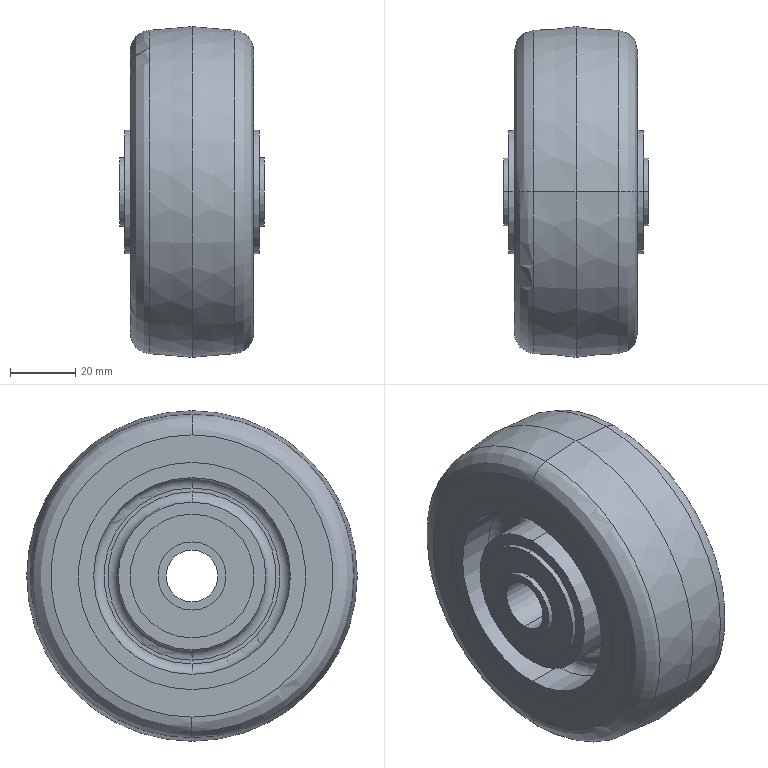Part | SolidWorks | features Revolution 1 | 1 solid | 56 faces | box 44.45 x 101.6 x 101.6 mm | volume 249789 mm3 | cylinder 26 | plane 14 | torus 12 | cone 4 | commonest cylinder face diameters 15.85 x4 20.955 x4 38.1 x4 45.415 x4 60.452 x4 69.85 x4
STEP:
#1=CARTESIAN_POINT('',(-0.375,0.,-0.312));
#2=VERTEX_POINT('',#1);
#3=CARTESIAN_POINT('',(-0.375,0.,0.312));
#4=VERTEX_POINT('',#3);
#5=CARTESIAN_POINT('',(-0.375,0.,0.));
#6=DIRECTION('',(-1.,0.,0.));
#7=DIRECTION('',(0.,0.,1.));
#8=AXIS2_PLACEMENT_3D('',#5,#6,#7);
#9=CIRCLE('',#8,0.312);
#10=EDGE_CURVE('',#2,#4,#9,.T.);
#11=ORIENTED_EDGE('',*,*,#10,.F.);
#12=CARTESIAN_POINT('',(-0.875,0.,-0.312));
#13=VERTEX_POINT('',#12);
#14=CARTESIAN_POINT('',(-1.26,0.,-0.312));
#15=DIRECTION('',(-1.,0.,0.));
#16=VECTOR('',#15,39.37);
#17=LINE('',#14,#16);
#18=EDGE_CURVE('',#2,#13,#17,.T.);
#19=ORIENTED_EDGE('',*,*,#18,.T.);
#20=CARTESIAN_POINT('',(-0.875,0.,0.312));
#21=VERTEX_POINT('',#20);
#22=CARTESIAN_POINT('',(-0.875,0.,0.));
#23=DIRECTION('',(-1.,0.,0.));
#24=DIRECTION('',(0.,0.,1.));
#25=AXIS2_PLACEMENT_3D('',#22,#23,#24);
#26=CIRCLE('',#25,0.312);
#27=EDGE_CURVE('',#13,#21,#26,.T.);
#28=ORIENTED_EDGE('',*,*,#27,.T.);
#29=CARTESIAN_POINT('',(-1.26,0.,0.312));
#30=DIRECTION('',(-1.,0.,0.));
#31=VECTOR('',#30,39.37);
#32=LINE('',#29,#31);
#33=EDGE_CURVE('',#4,#21,#32,.T.);
#34=ORIENTED_EDGE('',*,*,#33,.F.);
#35=EDGE_LOOP('',(#11,#19,#28,#34));
#36=FACE_OUTER_BOUND('',#35,.T.);
#37=CARTESIAN_POINT('',(-1.26,0.,0.));
#38=DIRECTION('',(-1.,0.,0.));
#39=DIRECTION('',(0.,0.,1.));
#40=AXIS2_PLACEMENT_3D('',#37,#38,#39);
#41=CYLINDRICAL_SURFACE('',#40,0.312);
#42=ADVANCED_FACE('',(#36),#41,.F.);
#43=CARTESIAN_POINT('',(-0.8125,0.,0.4125));
#44=VERTEX_POINT('',#43);
#45=CARTESIAN_POINT('',(-0.8125,0.,-0.4125));
#46=VERTEX_POINT('',#45);
#47=CARTESIAN_POINT('',(-0.8125,0.,0.));
#48=DIRECTION('',(-1.,0.,0.));
#49=DIRECTION('',(0.,0.,1.));
#50=AXIS2_PLACEMENT_3D('',#47,#48,#49);
#51=CIRCLE('',#50,0.4125);
#52=EDGE_CURVE('',#44,#46,#51,.T.);
#53=ORIENTED_EDGE('',*,*,#52,.T.);
#54=CARTESIAN_POINT('',(-0.875,0.,-0.4125));
#55=VERTEX_POINT('',#54);
#56=CARTESIAN_POINT('',(-1.26,0.,-0.4125));
#57=DIRECTION('',(-1.,0.,0.));
#58=VECTOR('',#57,39.37);
#59=LINE('',#56,#58);
#60=EDGE_CURVE('',#46,#55,#59,.T.);
#61=ORIENTED_EDGE('',*,*,#60,.T.);
#62=CARTESIAN_POINT('',(-0.875,0.,0.4125));
#63=VERTEX_POINT('',#62);
#64=CARTESIAN_POINT('',(-0.875,0.,0.));
#65=DIRECTION('',(-1.,0.,0.));
#66=DIRECTION('',(0.,0.,1.));
#67=AXIS2_PLACEMENT_3D('',#64,#65,#66);
#68=CIRCLE('',#67,0.4125);
#69=EDGE_CURVE('',#63,#55,#68,.T.);
#70=ORIENTED_EDGE('',*,*,#69,.F.);
#71=CARTESIAN_POINT('',(-1.26,0.,0.4125));
#72=DIRECTION('',(-1.,0.,0.));
#73=VECTOR('',#72,39.37);
#74=LINE('',#71,#73);
#75=EDGE_CURVE('',#44,#63,#74,.T.);
#76=ORIENTED_EDGE('',*,*,#75,.F.);
#77=EDGE_LOOP('',(#53,#61,#70,#76));
#78=FACE_OUTER_BOUND('',#77,.T.);
#79=CARTESIAN_POINT('',(-1.26,0.,0.));
#80=DIRECTION('',(-1.,0.,0.));
#81=DIRECTION('',(0.,0.,1.));
#82=AXIS2_PLACEMENT_3D('',#79,#80,#81);
#83=CYLINDRICAL_SURFACE('',#82,0.4125);
#84=ADVANCED_FACE('',(#78),#83,.T.);
#85=CARTESIAN_POINT('',(-0.75,0.,0.75));
#86=VERTEX_POINT('',#85);
#87=CARTESIAN_POINT('',(-0.75,0.,-0.75));
#88=VERTEX_POINT('',#87);
#89=CARTESIAN_POINT('',(-0.75,0.,0.));
#90=DIRECTION('',(-1.,0.,0.));
#91=DIRECTION('',(0.,0.,1.));
#92=AXIS2_PLACEMENT_3D('',#89,#90,#91);
#93=CIRCLE('',#92,0.75);
#94=EDGE_CURVE('',#86,#88,#93,.T.);
#95=ORIENTED_EDGE('',*,*,#94,.T.);
#96=CARTESIAN_POINT('',(-0.8125,0.,-0.75));
#97=VERTEX_POINT('',#96);
#98=CARTESIAN_POINT('',(-1.26,0.,-0.75));
#99=DIRECTION('',(-1.,0.,0.));
#100=VECTOR('',#99,39.37);
#101=LINE('',#98,#100);
#102=EDGE_CURVE('',#88,#97,#101,.T.);
#103=ORIENTED_EDGE('',*,*,#102,.T.);
#104=CARTESIAN_POINT('',(-0.8125,0.,0.75));
#105=VERTEX_POINT('',#104);
#106=CARTESIAN_POINT('',(-0.8125,0.,0.));
#107=DIRECTION('',(-1.,0.,0.));
#108=DIRECTION('',(0.,0.,1.));
#109=AXIS2_PLACEMENT_3D('',#106,#107,#108);
#110=CIRCLE('',#109,0.75);
#111=EDGE_CURVE('',#105,#97,#110,.T.);
#112=ORIENTED_EDGE('',*,*,#111,.F.);
#113=CARTESIAN_POINT('',(-1.26,0.,0.75));
#114=DIRECTION('',(-1.,0.,0.));
#115=VECTOR('',#114,39.37);
#116=LINE('',#113,#115);
#117=EDGE_CURVE('',#86,#105,#116,.T.);
#118=ORIENTED_EDGE('',*,*,#117,.F.);
#119=EDGE_LOOP('',(#95,#103,#112,#118));
#120=FACE_OUTER_BOUND('',#119,.T.);
#121=CARTESIAN_POINT('',(-1.26,0.,0.));
#122=DIRECTION('',(-1.,0.,0.));
#123=DIRECTION('',(0.,0.,1.));
#124=AXIS2_PLACEMENT_3D('',#121,#122,#123);
#125=CYLINDRICAL_SURFACE('',#124,0.75);
#126=ADVANCED_FACE('',(#120),#125,.T.);
#127=CARTESIAN_POINT('',(-0.3125,0.,0.894));
#128=VERTEX_POINT('',#127);
#129=CARTESIAN_POINT('',(-0.3125,0.,-0.894));
#130=VERTEX_POINT('',#129);
#131=CARTESIAN_POINT('',(-0.3125,0.,0.));
#132=DIRECTION('',(-1.,0.,0.));
#133=DIRECTION('',(0.,0.,1.));
#134=AXIS2_PLACEMENT_3D('',#131,#132,#133);
#135=CIRCLE('',#134,0.894);
#136=EDGE_CURVE('',#128,#130,#135,.T.);
#137=ORIENTED_EDGE('',*,*,#136,.T.);
#138=CARTESIAN_POINT('',(-0.75,0.,-0.894));
#139=VERTEX_POINT('',#138);
#140=CARTESIAN_POINT('',(-1.26,0.,-0.894));
#141=DIRECTION('',(-1.,0.,0.));
#142=VECTOR('',#141,39.37);
#143=LINE('',#140,#142);
#144=EDGE_CURVE('',#130,#139,#143,.T.);
#145=ORIENTED_EDGE('',*,*,#144,.T.);
#146=CARTESIAN_POINT('',(-0.75,0.,0.894));
#147=VERTEX_POINT('',#146);
#148=CARTESIAN_POINT('',(-0.75,0.,0.));
#149=DIRECTION('',(-1.,0.,0.));
#150=DIRECTION('',(0.,0.,1.));
#151=AXIS2_PLACEMENT_3D('',#148,#149,#150);
#152=CIRCLE('',#151,0.894);
#153=EDGE_CURVE('',#147,#139,#152,.T.);
#154=ORIENTED_EDGE('',*,*,#153,.F.);
#155=CARTESIAN_POINT('',(-1.26,0.,0.894));
#156=DIRECTION('',(-1.,0.,0.));
#157=VECTOR('',#156,39.37);
#158=LINE('',#155,#157);
#159=EDGE_CURVE('',#128,#147,#158,.T.);
#160=ORIENTED_EDGE('',*,*,#159,.F.);
#161=EDGE_LOOP('',(#137,#145,#154,#160));
#162=FACE_OUTER_BOUND('',#161,.T.);
#163=CARTESIAN_POINT('',(-1.26,0.,0.));
#164=DIRECTION('',(-1.,0.,0.));
#165=DIRECTION('',(0.,0.,1.));
#166=AXIS2_PLACEMENT_3D('',#163,#164,#165);
#167=CYLINDRICAL_SURFACE('',#166,0.894);
#168=ADVANCED_FACE('',(#162),#167,.T.);
#169=CARTESIAN_POINT('',(-0.3125,0.,0.));
#170=DIRECTION('',(-1.,0.,0.));
#171=DIRECTION('',(0.,0.,1.));
#172=AXIS2_PLACEMENT_3D('',#169,#170,#171);
#173=CIRCLE('',#172,0.894);
#174=EDGE_CURVE('',#130,#128,#173,.T.);
#175=ORIENTED_EDGE('',*,*,#174,.F.);
#176=CARTESIAN_POINT('',(-0.1875,0.,-1.019));
#177=VERTEX_POINT('',#176);
#178=CARTESIAN_POINT('',(-0.3125,0.,-1.019));
#179=DIRECTION('',(0.,1.,0.));
#180=DIRECTION('',(0.,0.,1.));
#181=AXIS2_PLACEMENT_3D('',#178,#179,#180);
#182=CIRCLE('',#181,0.125);
#183=EDGE_CURVE('',#130,#177,#182,.T.);
#184=ORIENTED_EDGE('',*,*,#183,.T.);
#185=CARTESIAN_POINT('',(-0.1875,0.,1.019));
#186=VERTEX_POINT('',#185);
#187=CARTESIAN_POINT('',(-0.1875,0.,0.));
#188=DIRECTION('',(-1.,0.,0.));
#189=DIRECTION('',(0.,0.,1.));
#190=AXIS2_PLACEMENT_3D('',#187,#188,#189);
#191=CIRCLE('',#190,1.019);
#192=EDGE_CURVE('',#177,#186,#191,.T.);
#193=ORIENTED_EDGE('',*,*,#192,.T.);
#194=CARTESIAN_POINT('',(-0.3125,0.,1.019));
#195=DIRECTION('',(0.,-1.,0.));
#196=DIRECTION('',(0.,0.,-1.));
#197=AXIS2_PLACEMENT_3D('',#194,#195,#196);
#198=CIRCLE('',#197,0.125);
#199=EDGE_CURVE('',#128,#186,#198,.T.);
#200=ORIENTED_EDGE('',*,*,#199,.F.);
#201=EDGE_LOOP('',(#175,#184,#193,#200));
#202=FACE_OUTER_BOUND('',#201,.T.);
#203=CARTESIAN_POINT('',(-0.3125,0.,0.));
#204=DIRECTION('',(-1.,0.,0.));
#205=DIRECTION('',(0.,0.,1.));
#206=AXIS2_PLACEMENT_3D('',#203,#204,#205);
#207=TOROIDAL_SURFACE('',#206,1.019,0.125);
#208=ADVANCED_FACE('',(#202),#207,.F.);
#209=CARTESIAN_POINT('',(-0.1875,0.,-1.065));
#210=VERTEX_POINT('',#209);
#211=CARTESIAN_POINT('',(-0.1875,0.,1.065));
#212=VERTEX_POINT('',#211);
#213=CARTESIAN_POINT('',(-0.1875,0.,0.));
#214=DIRECTION('',(-1.,0.,0.));
#215=DIRECTION('',(0.,0.,1.));
#216=AXIS2_PLACEMENT_3D('',#213,#214,#215);
#217=CIRCLE('',#216,1.065);
#218=EDGE_CURVE('',#210,#212,#217,.T.);
#219=ORIENTED_EDGE('',*,*,#218,.F.);
#220=CARTESIAN_POINT('',(-0.3125,0.,-1.19));
#221=VERTEX_POINT('',#220);
#222=CARTESIAN_POINT('',(-0.3125,0.,-1.065));
#223=DIRECTION('',(0.,1.,0.));
#224=DIRECTION('',(0.,0.,1.));
#225=AXIS2_PLACEMENT_3D('',#222,#223,#224);
#226=CIRCLE('',#225,0.125);
#227=EDGE_CURVE('',#210,#221,#226,.T.);
#228=ORIENTED_EDGE('',*,*,#227,.T.);
#229=CARTESIAN_POINT('',(-0.3125,0.,1.19));
#230=VERTEX_POINT('',#229);
#231=CARTESIAN_POINT('',(-0.3125,0.,0.));
#232=DIRECTION('',(-1.,0.,0.));
#233=DIRECTION('',(0.,0.,1.));
#234=AXIS2_PLACEMENT_3D('',#231,#232,#233);
#235=CIRCLE('',#234,1.19);
#236=EDGE_CURVE('',#221,#230,#235,.T.);
#237=ORIENTED_EDGE('',*,*,#236,.T.);
#238=CARTESIAN_POINT('',(-0.3125,0.,1.065));
#239=DIRECTION('',(0.,-1.,0.));
#240=DIRECTION('',(0.,0.,-1.));
#241=AXIS2_PLACEMENT_3D('',#238,#239,#240);
#242=CIRCLE('',#241,0.125);
#243=EDGE_CURVE('',#212,#230,#242,.T.);
#244=ORIENTED_EDGE('',*,*,#243,.F.);
#245=EDGE_LOOP('',(#219,#228,#237,#244));
#246=FACE_OUTER_BOUND('',#245,.T.);
#247=CARTESIAN_POINT('',(-0.3125,0.,0.));
#248=DIRECTION('',(-1.,0.,0.));
#249=DIRECTION('',(0.,0.,1.));
#250=AXIS2_PLACEMENT_3D('',#247,#248,#249);
#251=TOROIDAL_SURFACE('',#250,1.065,0.125);
#252=ADVANCED_FACE('',(#246),#251,.F.);
#253=ORIENTED_EDGE('',*,*,#236,.F.);
#254=CARTESIAN_POINT('',(-0.75,0.,-1.19));
#255=VERTEX_POINT('',#254);
#256=CARTESIAN_POINT('',(-1.26,0.,-1.19));
#257=DIRECTION('',(-1.,0.,0.));
#258=VECTOR('',#257,39.37);
#259=LINE('',#256,#258);
#260=EDGE_CURVE('',#221,#255,#259,.T.);
#261=ORIENTED_EDGE('',*,*,#260,.T.);
#262=CARTESIAN_POINT('',(-0.75,0.,1.19));
#263=VERTEX_POINT('',#262);
#264=CARTESIAN_POINT('',(-0.75,0.,0.));
#265=DIRECTION('',(-1.,0.,0.));
#266=DIRECTION('',(0.,0.,1.));
#267=AXIS2_PLACEMENT_3D('',#264,#265,#266);
#268=CIRCLE('',#267,1.19);
#269=EDGE_CURVE('',#255,#263,#268,.T.);
#270=ORIENTED_EDGE('',*,*,#269,.T.);
#271=CARTESIAN_POINT('',(-1.26,0.,1.19));
#272=DIRECTION('',(-1.,0.,0.));
#273=VECTOR('',#272,39.37);
#274=LINE('',#271,#273);
#275=EDGE_CURVE('',#230,#263,#274,.T.);
#276=ORIENTED_EDGE('',*,*,#275,.F.);
#277=EDGE_LOOP('',(#253,#261,#270,#276));
#278=FACE_OUTER_BOUND('',#277,.T.);
#279=CARTESIAN_POINT('',(-1.26,0.,0.));
#280=DIRECTION('',(-1.,0.,0.));
#281=DIRECTION('',(0.,0.,1.));
#282=AXIS2_PLACEMENT_3D('',#279,#280,#281);
#283=CYLINDRICAL_SURFACE('',#282,1.19);
#284=ADVANCED_FACE('',(#278),#283,.F.);
#285=CARTESIAN_POINT('',(-0.745,0.,1.375));
#286=VERTEX_POINT('',#285);
#287=CARTESIAN_POINT('',(-0.745,0.,-1.375));
#288=VERTEX_POINT('',#287);
#289=CARTESIAN_POINT('',(-0.745,0.,0.));
#290=DIRECTION('',(-1.,0.,0.));
#291=DIRECTION('',(0.,0.,1.));
#292=AXIS2_PLACEMENT_3D('',#289,#290,#291);
#293=CIRCLE('',#292,1.375);
#294=EDGE_CURVE('',#286,#288,#293,.T.);
#295=ORIENTED_EDGE('',*,*,#294,.T.);
#296=CARTESIAN_POINT('',(-0.75,0.,-1.375));
#297=VERTEX_POINT('',#296);
#298=CARTESIAN_POINT('',(-1.26,0.,-1.375));
#299=DIRECTION('',(-1.,0.,0.));
#300=VECTOR('',#299,39.37);
#301=LINE('',#298,#300);
#302=EDGE_CURVE('',#288,#297,#301,.T.);
#303=ORIENTED_EDGE('',*,*,#302,.T.);
#304=CARTESIAN_POINT('',(-0.75,0.,1.375));
#305=VERTEX_POINT('',#304);
#306=CARTESIAN_POINT('',(-0.75,0.,0.));
#307=DIRECTION('',(-1.,0.,0.));
#308=DIRECTION('',(0.,0.,1.));
#309=AXIS2_PLACEMENT_3D('',#306,#307,#308);
#310=CIRCLE('',#309,1.375);
#311=EDGE_CURVE('',#305,#297,#310,.T.);
#312=ORIENTED_EDGE('',*,*,#311,.F.);
#313=CARTESIAN_POINT('',(-1.26,0.,1.375));
#314=DIRECTION('',(-1.,0.,0.));
#315=VECTOR('',#314,39.37);
#316=LINE('',#313,#315);
#317=EDGE_CURVE('',#286,#305,#316,.T.);
#318=ORIENTED_EDGE('',*,*,#317,.F.);
#319=EDGE_LOOP('',(#295,#303,#312,#318));
#320=FACE_OUTER_BOUND('',#319,.T.);
#321=CARTESIAN_POINT('',(-1.26,0.,0.));
#322=DIRECTION('',(-1.,0.,0.));
#323=DIRECTION('',(0.,0.,1.));
#324=AXIS2_PLACEMENT_3D('',#321,#322,#323);
#325=CYLINDRICAL_SURFACE('',#324,1.375);
#326=ADVANCED_FACE('',(#320),#325,.T.);
#327=CARTESIAN_POINT('',(-0.5159,0.,1.957));
#328=VERTEX_POINT('',#327);
#329=CARTESIAN_POINT('',(-0.5159,0.,-1.957));
#330=VERTEX_POINT('',#329);
#331=CARTESIAN_POINT('',(-0.5159,0.,0.));
#332=DIRECTION('',(-1.,0.,0.));
#333=DIRECTION('',(0.,0.,1.));
#334=AXIS2_PLACEMENT_3D('',#331,#332,#333);
#335=CIRCLE('',#334,1.957);
#336=EDGE_CURVE('',#328,#330,#335,.T.);
#337=ORIENTED_EDGE('',*,*,#336,.T.);
#338=CARTESIAN_POINT('',(-0.745,0.,-1.708));
#339=VERTEX_POINT('',#338);
#340=CARTESIAN_POINT('',(-0.495,0.,-1.708));
#341=DIRECTION('',(0.,1.,0.));
#342=DIRECTION('',(0.,0.,1.));
#343=AXIS2_PLACEMENT_3D('',#340,#341,#342);
#344=CIRCLE('',#343,0.25);
#345=EDGE_CURVE('',#330,#339,#344,.T.);
#346=ORIENTED_EDGE('',*,*,#345,.T.);
#347=CARTESIAN_POINT('',(-0.745,0.,1.708));
#348=VERTEX_POINT('',#347);
#349=CARTESIAN_POINT('',(-0.745,0.,0.));
#350=DIRECTION('',(-1.,0.,0.));
#351=DIRECTION('',(0.,0.,1.));
#352=AXIS2_PLACEMENT_3D('',#349,#350,#351);
#353=CIRCLE('',#352,1.708);
#354=EDGE_CURVE('',#348,#339,#353,.T.);
#355=ORIENTED_EDGE('',*,*,#354,.F.);
#356=CARTESIAN_POINT('',(-0.495,0.,1.708));
#357=DIRECTION('',(0.,-1.,0.));
#358=DIRECTION('',(0.,0.,-1.));
#359=AXIS2_PLACEMENT_3D('',#356,#357,#358);
#360=CIRCLE('',#359,0.25);
#361=EDGE_CURVE('',#328,#348,#360,.T.);
#362=ORIENTED_EDGE('',*,*,#361,.F.);
#363=EDGE_LOOP('',(#337,#346,#355,#362));
#364=FACE_OUTER_BOUND('',#363,.T.);
#365=CARTESIAN_POINT('',(-0.495,0.,0.));
#366=DIRECTION('',(-1.,0.,0.));
#367=DIRECTION('',(0.,0.,1.));
#368=AXIS2_PLACEMENT_3D('',#365,#366,#367);
#369=TOROIDAL_SURFACE('',#368,1.708,0.25);
#370=ADVANCED_FACE('',(#364),#369,.T.);
#371=ORIENTED_EDGE('',*,*,#336,.F.);
#372=CARTESIAN_POINT('',(0.,0.,2.));
#373=VERTEX_POINT('',#372);
#374=CARTESIAN_POINT('',(0.,0.,2.));
#375=DIRECTION('',(0.9965,0.,0.08363));
#376=VECTOR('',#375,39.37);
#377=LINE('',#374,#376);
#378=EDGE_CURVE('',#328,#373,#377,.T.);
#379=ORIENTED_EDGE('',*,*,#378,.T.);
#380=CARTESIAN_POINT('',(0.,0.,-2.));
#381=VERTEX_POINT('',#380);
#382=CARTESIAN_POINT('',(0.,0.,0.));
#383=DIRECTION('',(-1.,0.,0.));
#384=DIRECTION('',(0.,0.,1.));
#385=AXIS2_PLACEMENT_3D('',#382,#383,#384);
#386=CIRCLE('',#385,2.);
#387=EDGE_CURVE('',#373,#381,#386,.T.);
#388=ORIENTED_EDGE('',*,*,#387,.T.);
#389=CARTESIAN_POINT('',(0.,0.,-2.));
#390=DIRECTION('',(0.9965,0.,-0.08363));
#391=VECTOR('',#390,39.37);
#392=LINE('',#389,#391);
#393=EDGE_CURVE('',#330,#381,#392,.T.);
#394=ORIENTED_EDGE('',*,*,#393,.F.);
#395=EDGE_LOOP('',(#371,#379,#388,#394));
#396=FACE_OUTER_BOUND('',#395,.T.);
#397=CARTESIAN_POINT('',(0.,0.,0.));
#398=DIRECTION('',(1.,0.,0.));
#399=DIRECTION('',(0.,0.,-1.));
#400=AXIS2_PLACEMENT_3D('',#397,#398,#399);
#401=CONICAL_SURFACE('',#400,2.,0.08373);
#402=ADVANCED_FACE('',(#396),#401,.T.);
#403=CARTESIAN_POINT('',(0.5159,0.,1.957));
#404=VERTEX_POINT('',#403);
#405=CARTESIAN_POINT('',(0.5159,0.,-1.957));
#406=VERTEX_POINT('',#405);
#407=CARTESIAN_POINT('',(0.5159,0.,0.));
#408=DIRECTION('',(-1.,0.,0.));
#409=DIRECTION('',(0.,0.,1.));
#410=AXIS2_PLACEMENT_3D('',#407,#408,#409);
#411=CIRCLE('',#410,1.957);
#412=EDGE_CURVE('',#404,#406,#411,.T.);
#413=ORIENTED_EDGE('',*,*,#412,.T.);
#414=CARTESIAN_POINT('',(0.5159,0.,-1.957));
#415=DIRECTION('',(-0.9965,0.,-0.08363));
#416=VECTOR('',#415,39.37);
#417=LINE('',#414,#416);
#418=EDGE_CURVE('',#406,#381,#417,.T.);
#419=ORIENTED_EDGE('',*,*,#418,.T.);
#420=ORIENTED_EDGE('',*,*,#387,.F.);
#421=CARTESIAN_POINT('',(0.5159,0.,1.957));
#422=DIRECTION('',(-0.9965,0.,0.08363));
#423=VECTOR('',#422,39.37);
#424=LINE('',#421,#423);
#425=EDGE_CURVE('',#404,#373,#424,.T.);
#426=ORIENTED_EDGE('',*,*,#425,.F.);
#427=EDGE_LOOP('',(#413,#419,#420,#426));
#428=FACE_OUTER_BOUND('',#427,.T.);
#429=CARTESIAN_POINT('',(0.5159,0.,0.));
#430=DIRECTION('',(-1.,0.,0.));
#431=DIRECTION('',(0.,0.,1.));
#432=AXIS2_PLACEMENT_3D('',#429,#430,#431);
#433=CONICAL_SURFACE('',#432,1.957,0.08373);
#434=ADVANCED_FACE('',(#428),#433,.T.);
#435=CARTESIAN_POINT('',(0.745,0.,1.708));
#436=VERTEX_POINT('',#435);
#437=CARTESIAN_POINT('',(0.745,0.,-1.708));
#438=VERTEX_POINT('',#437);
#439=CARTESIAN_POINT('',(0.745,0.,0.));
#440=DIRECTION('',(-1.,0.,0.));
#441=DIRECTION('',(0.,0.,1.));
#442=AXIS2_PLACEMENT_3D('',#439,#440,#441);
#443=CIRCLE('',#442,1.708);
#444=EDGE_CURVE('',#436,#438,#443,.T.);
#445=ORIENTED_EDGE('',*,*,#444,.T.);
#446=CARTESIAN_POINT('',(0.495,0.,-1.708));
#447=DIRECTION('',(0.,1.,0.));
#448=DIRECTION('',(0.,0.,1.));
#449=AXIS2_PLACEMENT_3D('',#446,#447,#448);
#450=CIRCLE('',#449,0.25);
#451=EDGE_CURVE('',#438,#406,#450,.T.);
#452=ORIENTED_EDGE('',*,*,#451,.T.);
#453=ORIENTED_EDGE('',*,*,#412,.F.);
#454=CARTESIAN_POINT('',(0.495,0.,1.708));
#455=DIRECTION('',(0.,-1.,0.));
#456=DIRECTION('',(0.,0.,-1.));
#457=AXIS2_PLACEMENT_3D('',#454,#455,#456);
#458=CIRCLE('',#457,0.25);
#459=EDGE_CURVE('',#436,#404,#458,.T.);
#460=ORIENTED_EDGE('',*,*,#459,.F.);
#461=EDGE_LOOP('',(#445,#452,#453,#460));
#462=FACE_OUTER_BOUND('',#461,.T.);
#463=CARTESIAN_POINT('',(0.495,0.,0.));
#464=DIRECTION('',(-1.,0.,0.));
#465=DIRECTION('',(0.,0.,1.));
#466=AXIS2_PLACEMENT_3D('',#463,#464,#465);
#467=TOROIDAL_SURFACE('',#466,1.708,0.25);
#468=ADVANCED_FACE('',(#462),#467,.T.);
#469=CARTESIAN_POINT('',(0.75,0.,1.375));
#470=VERTEX_POINT('',#469);
#471=CARTESIAN_POINT('',(0.75,0.,-1.375));
#472=VERTEX_POINT('',#471);
#473=CARTESIAN_POINT('',(0.75,0.,0.));
#474=DIRECTION('',(-1.,0.,0.));
#475=DIRECTION('',(0.,0.,1.));
#476=AXIS2_PLACEMENT_3D('',#473,#474,#475);
#477=CIRCLE('',#476,1.375);
#478=EDGE_CURVE('',#470,#472,#477,.T.);
#479=ORIENTED_EDGE('',*,*,#478,.T.);
#480=CARTESIAN_POINT('',(0.745,0.,-1.375));
#481=VERTEX_POINT('',#480);
#482=CARTESIAN_POINT('',(-1.26,0.,-1.375));
#483=DIRECTION('',(-1.,0.,0.));
#484=VECTOR('',#483,39.37);
#485=LINE('',#482,#484);
#486=EDGE_CURVE('',#472,#481,#485,.T.);
#487=ORIENTED_EDGE('',*,*,#486,.T.);
#488=CARTESIAN_POINT('',(0.745,0.,1.375));
#489=VERTEX_POINT('',#488);
#490=CARTESIAN_POINT('',(0.745,0.,0.));
#491=DIRECTION('',(-1.,0.,0.));
#492=DIRECTION('',(0.,0.,1.));
#493=AXIS2_PLACEMENT_3D('',#490,#491,#492);
#494=CIRCLE('',#493,1.375);
#495=EDGE_CURVE('',#489,#481,#494,.T.);
#496=ORIENTED_EDGE('',*,*,#495,.F.);
#497=CARTESIAN_POINT('',(-1.26,0.,1.375));
#498=DIRECTION('',(-1.,0.,0.));
#499=VECTOR('',#498,39.37);
#500=LINE('',#497,#499);
#501=EDGE_CURVE('',#470,#489,#500,.T.);
#502=ORIENTED_EDGE('',*,*,#501,.F.);
#503=EDGE_LOOP('',(#479,#487,#496,#502));
#504=FACE_OUTER_BOUND('',#503,.T.);
#505=CARTESIAN_POINT('',(-1.26,0.,0.));
#506=DIRECTION('',(-1.,0.,0.));
#507=DIRECTION('',(0.,0.,1.));
#508=AXIS2_PLACEMENT_3D('',#505,#506,#507);
#509=CYLINDRICAL_SURFACE('',#508,1.375);
#510=ADVANCED_FACE('',(#504),#509,.T.);
#511=CARTESIAN_POINT('',(0.75,0.,-1.19));
#512=VERTEX_POINT('',#511);
#513=CARTESIAN_POINT('',(0.75,0.,1.19));
#514=VERTEX_POINT('',#513);
#515=CARTESIAN_POINT('',(0.75,0.,0.));
#516=DIRECTION('',(-1.,0.,0.));
#517=DIRECTION('',(0.,0.,1.));
#518=AXIS2_PLACEMENT_3D('',#515,#516,#517);
#519=CIRCLE('',#518,1.19);
#520=EDGE_CURVE('',#512,#514,#519,.T.);
#521=ORIENTED_EDGE('',*,*,#520,.F.);
#522=CARTESIAN_POINT('',(0.3125,0.,-1.19));
#523=VERTEX_POINT('',#522);
#524=CARTESIAN_POINT('',(-1.26,0.,-1.19));
#525=DIRECTION('',(-1.,0.,0.));
#526=VECTOR('',#525,39.37);
#527=LINE('',#524,#526);
#528=EDGE_CURVE('',#512,#523,#527,.T.);
#529=ORIENTED_EDGE('',*,*,#528,.T.);
#530=CARTESIAN_POINT('',(0.3125,0.,1.19));
#531=VERTEX_POINT('',#530);
#532=CARTESIAN_POINT('',(0.3125,0.,0.));
#533=DIRECTION('',(-1.,0.,0.));
#534=DIRECTION('',(0.,0.,1.));
#535=AXIS2_PLACEMENT_3D('',#532,#533,#534);
#536=CIRCLE('',#535,1.19);
#537=EDGE_CURVE('',#523,#531,#536,.T.);
#538=ORIENTED_EDGE('',*,*,#537,.T.);
#539=CARTESIAN_POINT('',(-1.26,0.,1.19));
#540=DIRECTION('',(-1.,0.,0.));
#541=VECTOR('',#540,39.37);
#542=LINE('',#539,#541);
#543=EDGE_CURVE('',#514,#531,#542,.T.);
#544=ORIENTED_EDGE('',*,*,#543,.F.);
#545=EDGE_LOOP('',(#521,#529,#538,#544));
#546=FACE_OUTER_BOUND('',#545,.T.);
#547=CARTESIAN_POINT('',(-1.26,0.,0.));
#548=DIRECTION('',(-1.,0.,0.));
#549=DIRECTION('',(0.,0.,1.));
#550=AXIS2_PLACEMENT_3D('',#547,#548,#549);
#551=CYLINDRICAL_SURFACE('',#550,1.19);
#552=ADVANCED_FACE('',(#546),#551,.F.);
#553=ORIENTED_EDGE('',*,*,#537,.F.);
#554=CARTESIAN_POINT('',(0.1875,0.,-1.065));
#555=VERTEX_POINT('',#554);
#556=CARTESIAN_POINT('',(0.3125,0.,-1.065));
#557=DIRECTION('',(0.,1.,0.));
#558=DIRECTION('',(0.,0.,1.));
#559=AXIS2_PLACEMENT_3D('',#556,#557,#558);
#560=CIRCLE('',#559,0.125);
#561=EDGE_CURVE('',#523,#555,#560,.T.);
#562=ORIENTED_EDGE('',*,*,#561,.T.);
#563=CARTESIAN_POINT('',(0.1875,0.,1.065));
#564=VERTEX_POINT('',#563);
#565=CARTESIAN_POINT('',(0.1875,0.,0.));
#566=DIRECTION('',(-1.,0.,0.));
#567=DIRECTION('',(0.,0.,1.));
#568=AXIS2_PLACEMENT_3D('',#565,#566,#567);
#569=CIRCLE('',#568,1.065);
#570=EDGE_CURVE('',#555,#564,#569,.T.);
#571=ORIENTED_EDGE('',*,*,#570,.T.);
#572=CARTESIAN_POINT('',(0.3125,0.,1.065));
#573=DIRECTION('',(0.,-1.,0.));
#574=DIRECTION('',(0.,0.,-1.));
#575=AXIS2_PLACEMENT_3D('',#572,#573,#574);
#576=CIRCLE('',#575,0.125);
#577=EDGE_CURVE('',#531,#564,#576,.T.);
#578=ORIENTED_EDGE('',*,*,#577,.F.);
#579=EDGE_LOOP('',(#553,#562,#571,#578));
#580=FACE_OUTER_BOUND('',#579,.T.);
#581=CARTESIAN_POINT('',(0.3125,0.,0.));
#582=DIRECTION('',(-1.,0.,0.));
#583=DIRECTION('',(0.,0.,1.));
#584=AXIS2_PLACEMENT_3D('',#581,#582,#583);
#585=TOROIDAL_SURFACE('',#584,1.065,0.125);
#586=ADVANCED_FACE('',(#580),#585,.F.);
#587=CARTESIAN_POINT('',(0.1875,0.,-1.019));
#588=VERTEX_POINT('',#587);
#589=CARTESIAN_POINT('',(0.1875,0.,1.019));
#590=VERTEX_POINT('',#589);
#591=CARTESIAN_POINT('',(0.1875,0.,0.));
#592=DIRECTION('',(-1.,0.,0.));
#593=DIRECTION('',(0.,0.,1.));
#594=AXIS2_PLACEMENT_3D('',#591,#592,#593);
#595=CIRCLE('',#594,1.019);
#596=EDGE_CURVE('',#588,#590,#595,.T.);
#597=ORIENTED_EDGE('',*,*,#596,.F.);
#598=CARTESIAN_POINT('',(0.3125,0.,-0.894));
#599=VERTEX_POINT('',#598);
#600=CARTESIAN_POINT('',(0.3125,0.,-1.019));
#601=DIRECTION('',(0.,1.,0.));
#602=DIRECTION('',(0.,0.,1.));
#603=AXIS2_PLACEMENT_3D('',#600,#601,#602);
#604=CIRCLE('',#603,0.125);
#605=EDGE_CURVE('',#588,#599,#604,.T.);
#606=ORIENTED_EDGE('',*,*,#605,.T.);
#607=CARTESIAN_POINT('',(0.3125,0.,0.894));
#608=VERTEX_POINT('',#607);
#609=CARTESIAN_POINT('',(0.3125,0.,0.));
#610=DIRECTION('',(-1.,0.,0.));
#611=DIRECTION('',(0.,0.,1.));
#612=AXIS2_PLACEMENT_3D('',#609,#610,#611);
#613=CIRCLE('',#612,0.894);
#614=EDGE_CURVE('',#599,#608,#613,.T.);
#615=ORIENTED_EDGE('',*,*,#614,.T.);
#616=CARTESIAN_POINT('',(0.3125,0.,1.019));
#617=DIRECTION('',(0.,-1.,0.));
#618=DIRECTION('',(0.,0.,-1.));
#619=AXIS2_PLACEMENT_3D('',#616,#617,#618);
#620=CIRCLE('',#619,0.125);
#621=EDGE_CURVE('',#590,#608,#620,.T.);
#622=ORIENTED_EDGE('',*,*,#621,.F.);
#623=EDGE_LOOP('',(#597,#606,#615,#622));
#624=FACE_OUTER_BOUND('',#623,.T.);
#625=CARTESIAN_POINT('',(0.3125,0.,0.));
#626=DIRECTION('',(-1.,0.,0.));
#627=DIRECTION('',(0.,0.,1.));
#628=AXIS2_PLACEMENT_3D('',#625,#626,#627);
#629=TOROIDAL_SURFACE('',#628,1.019,0.125);
#630=ADVANCED_FACE('',(#624),#629,.F.);
#631=CARTESIAN_POINT('',(0.75,0.,0.894));
#632=VERTEX_POINT('',#631);
#633=CARTESIAN_POINT('',(0.75,0.,-0.894));
#634=VERTEX_POINT('',#633);
#635=CARTESIAN_POINT('',(0.75,0.,0.));
#636=DIRECTION('',(-1.,0.,0.));
#637=DIRECTION('',(0.,0.,1.));
#638=AXIS2_PLACEMENT_3D('',#635,#636,#637);
#639=CIRCLE('',#638,0.894);
#640=EDGE_CURVE('',#632,#634,#639,.T.);
#641=ORIENTED_EDGE('',*,*,#640,.T.);
#642=CARTESIAN_POINT('',(-1.26,0.,-0.894));
#643=DIRECTION('',(-1.,0.,0.));
#644=VECTOR('',#643,39.37);
#645=LINE('',#642,#644);
#646=EDGE_CURVE('',#634,#599,#645,.T.);
#647=ORIENTED_EDGE('',*,*,#646,.T.);
#648=CARTESIAN_POINT('',(0.3125,0.,0.));
#649=DIRECTION('',(-1.,0.,0.));
#650=DIRECTION('',(0.,0.,1.));
#651=AXIS2_PLACEMENT_3D('',#648,#649,#650);
#652=CIRCLE('',#651,0.894);
#653=EDGE_CURVE('',#608,#599,#652,.T.);
#654=ORIENTED_EDGE('',*,*,#653,.F.);
#655=CARTESIAN_POINT('',(-1.26,0.,0.894));
#656=DIRECTION('',(-1.,0.,0.));
#657=VECTOR('',#656,39.37);
#658=LINE('',#655,#657);
#659=EDGE_CURVE('',#632,#608,#658,.T.);
#660=ORIENTED_EDGE('',*,*,#659,.F.);
#661=EDGE_LOOP('',(#641,#647,#654,#660));
#662=FACE_OUTER_BOUND('',#661,.T.);
#663=CARTESIAN_POINT('',(-1.26,0.,0.));
#664=DIRECTION('',(-1.,0.,0.));
#665=DIRECTION('',(0.,0.,1.));
#666=AXIS2_PLACEMENT_3D('',#663,#664,#665);
#667=CYLINDRICAL_SURFACE('',#666,0.894);
#668=ADVANCED_FACE('',(#662),#667,.T.);
#669=CARTESIAN_POINT('',(0.8125,0.,0.75));
#670=VERTEX_POINT('',#669);
#671=CARTESIAN_POINT('',(0.8125,0.,-0.75));
#672=VERTEX_POINT('',#671);
#673=CARTESIAN_POINT('',(0.8125,0.,0.));
#674=DIRECTION('',(-1.,0.,0.));
#675=DIRECTION('',(0.,0.,1.));
#676=AXIS2_PLACEMENT_3D('',#673,#674,#675);
#677=CIRCLE('',#676,0.75);
#678=EDGE_CURVE('',#670,#672,#677,.T.);
#679=ORIENTED_EDGE('',*,*,#678,.T.);
#680=CARTESIAN_POINT('',(0.75,0.,-0.75));
#681=VERTEX_POINT('',#680);
#682=CARTESIAN_POINT('',(-1.26,0.,-0.75));
#683=DIRECTION('',(-1.,0.,0.));
#684=VECTOR('',#683,39.37);
#685=LINE('',#682,#684);
#686=EDGE_CURVE('',#672,#681,#685,.T.);
#687=ORIENTED_EDGE('',*,*,#686,.T.);
#688=CARTESIAN_POINT('',(0.75,0.,0.75));
#689=VERTEX_POINT('',#688);
#690=CARTESIAN_POINT('',(0.75,0.,0.));
#691=DIRECTION('',(-1.,0.,0.));
#692=DIRECTION('',(0.,0.,1.));
#693=AXIS2_PLACEMENT_3D('',#690,#691,#692);
#694=CIRCLE('',#693,0.75);
#695=EDGE_CURVE('',#689,#681,#694,.T.);
#696=ORIENTED_EDGE('',*,*,#695,.F.);
#697=CARTESIAN_POINT('',(-1.26,0.,0.75));
#698=DIRECTION('',(-1.,0.,0.));
#699=VECTOR('',#698,39.37);
#700=LINE('',#697,#699);
#701=EDGE_CURVE('',#670,#689,#700,.T.);
#702=ORIENTED_EDGE('',*,*,#701,.F.);
#703=EDGE_LOOP('',(#679,#687,#696,#702));
#704=FACE_OUTER_BOUND('',#703,.T.);
#705=CARTESIAN_POINT('',(-1.26,0.,0.));
#706=DIRECTION('',(-1.,0.,0.));
#707=DIRECTION('',(0.,0.,1.));
#708=AXIS2_PLACEMENT_3D('',#705,#706,#707);
#709=CYLINDRICAL_SURFACE('',#708,0.75);
#710=ADVANCED_FACE('',(#704),#709,.T.);
#711=CARTESIAN_POINT('',(0.875,0.,0.4125));
#712=VERTEX_POINT('',#711);
#713=CARTESIAN_POINT('',(0.875,0.,-0.4125));
#714=VERTEX_POINT('',#713);
#715=CARTESIAN_POINT('',(0.875,0.,0.));
#716=DIRECTION('',(-1.,0.,0.));
#717=DIRECTION('',(0.,0.,1.));
#718=AXIS2_PLACEMENT_3D('',#715,#716,#717);
#719=CIRCLE('',#718,0.4125);
#720=EDGE_CURVE('',#712,#714,#719,.T.);
#721=ORIENTED_EDGE('',*,*,#720,.T.);
#722=CARTESIAN_POINT('',(0.8125,0.,-0.4125));
#723=VERTEX_POINT('',#722);
#724=CARTESIAN_POINT('',(-1.26,0.,-0.4125));
#725=DIRECTION('',(-1.,0.,0.));
#726=VECTOR('',#725,39.37);
#727=LINE('',#724,#726);
#728=EDGE_CURVE('',#714,#723,#727,.T.);
#729=ORIENTED_EDGE('',*,*,#728,.T.);
#730=CARTESIAN_POINT('',(0.8125,0.,0.4125));
#731=VERTEX_POINT('',#730);
#732=CARTESIAN_POINT('',(0.8125,0.,0.));
#733=DIRECTION('',(-1.,0.,0.));
#734=DIRECTION('',(0.,0.,1.));
#735=AXIS2_PLACEMENT_3D('',#732,#733,#734);
#736=CIRCLE('',#735,0.4125);
#737=EDGE_CURVE('',#731,#723,#736,.T.);
#738=ORIENTED_EDGE('',*,*,#737,.F.);
#739=CARTESIAN_POINT('',(-1.26,0.,0.4125));
#740=DIRECTION('',(-1.,0.,0.));
#741=VECTOR('',#740,39.37);
#742=LINE('',#739,#741);
#743=EDGE_CURVE('',#712,#731,#742,.T.);
#744=ORIENTED_EDGE('',*,*,#743,.F.);
#745=EDGE_LOOP('',(#721,#729,#738,#744));
#746=FACE_OUTER_BOUND('',#745,.T.);
#747=CARTESIAN_POINT('',(-1.26,0.,0.));
#748=DIRECTION('',(-1.,0.,0.));
#749=DIRECTION('',(0.,0.,1.));
#750=AXIS2_PLACEMENT_3D('',#747,#748,#749);
#751=CYLINDRICAL_SURFACE('',#750,0.4125);
#752=ADVANCED_FACE('',(#746),#751,.T.);
#753=CARTESIAN_POINT('',(0.875,0.,-0.312));
#754=VERTEX_POINT('',#753);
#755=CARTESIAN_POINT('',(0.875,0.,0.312));
#756=VERTEX_POINT('',#755);
#757=CARTESIAN_POINT('',(0.875,0.,0.));
#758=DIRECTION('',(-1.,0.,0.));
#759=DIRECTION('',(0.,0.,1.));
#760=AXIS2_PLACEMENT_3D('',#757,#758,#759);
#761=CIRCLE('',#760,0.312);
#762=EDGE_CURVE('',#754,#756,#761,.T.);
#763=ORIENTED_EDGE('',*,*,#762,.F.);
#764=CARTESIAN_POINT('',(0.375,0.,-0.312));
#765=VERTEX_POINT('',#764);
#766=CARTESIAN_POINT('',(-1.26,0.,-0.312));
#767=DIRECTION('',(-1.,0.,0.));
#768=VECTOR('',#767,39.37);
#769=LINE('',#766,#768);
#770=EDGE_CURVE('',#754,#765,#769,.T.);
#771=ORIENTED_EDGE('',*,*,#770,.T.);
#772=CARTESIAN_POINT('',(0.375,0.,0.312));
#773=VERTEX_POINT('',#772);
#774=CARTESIAN_POINT('',(0.375,0.,0.));
#775=DIRECTION('',(-1.,0.,0.));
#776=DIRECTION('',(0.,0.,1.));
#777=AXIS2_PLACEMENT_3D('',#774,#775,#776);
#778=CIRCLE('',#777,0.312);
#779=EDGE_CURVE('',#765,#773,#778,.T.);
#780=ORIENTED_EDGE('',*,*,#779,.T.);
#781=CARTESIAN_POINT('',(-1.26,0.,0.312));
#782=DIRECTION('',(-1.,0.,0.));
#783=VECTOR('',#782,39.37);
#784=LINE('',#781,#783);
#785=EDGE_CURVE('',#756,#773,#784,.T.);
#786=ORIENTED_EDGE('',*,*,#785,.F.);
#787=EDGE_LOOP('',(#763,#771,#780,#786));
#788=FACE_OUTER_BOUND('',#787,.T.);
#789=CARTESIAN_POINT('',(-1.26,0.,0.));
#790=DIRECTION('',(-1.,0.,0.));
#791=DIRECTION('',(0.,0.,1.));
#792=AXIS2_PLACEMENT_3D('',#789,#790,#791);
#793=CYLINDRICAL_SURFACE('',#792,0.312);
#794=ADVANCED_FACE('',(#788),#793,.F.);
#795=CARTESIAN_POINT('',(0.375,0.,-0.5));
#796=VERTEX_POINT('',#795);
#797=CARTESIAN_POINT('',(0.375,0.,0.5));
#798=VERTEX_POINT('',#797);
#799=CARTESIAN_POINT('',(0.375,0.,0.));
#800=DIRECTION('',(-1.,0.,0.));
#801=DIRECTION('',(0.,0.,1.));
#802=AXIS2_PLACEMENT_3D('',#799,#800,#801);
#803=CIRCLE('',#802,0.5);
#804=EDGE_CURVE('',#796,#798,#803,.T.);
#805=ORIENTED_EDGE('',*,*,#804,.F.);
#806=CARTESIAN_POINT('',(-0.375,0.,-0.5));
#807=VERTEX_POINT('',#806);
#808=CARTESIAN_POINT('',(-1.26,0.,-0.5));
#809=DIRECTION('',(-1.,0.,0.));
#810=VECTOR('',#809,39.37);
#811=LINE('',#808,#810);
#812=EDGE_CURVE('',#796,#807,#811,.T.);
#813=ORIENTED_EDGE('',*,*,#812,.T.);
#814=CARTESIAN_POINT('',(-0.375,0.,0.5));
#815=VERTEX_POINT('',#814);
#816=CARTESIAN_POINT('',(-0.375,0.,0.));
#817=DIRECTION('',(-1.,0.,0.));
#818=DIRECTION('',(0.,0.,1.));
#819=AXIS2_PLACEMENT_3D('',#816,#817,#818);
#820=CIRCLE('',#819,0.5);
#821=EDGE_CURVE('',#807,#815,#820,.T.);
#822=ORIENTED_EDGE('',*,*,#821,.T.);
#823=CARTESIAN_POINT('',(-1.26,0.,0.5));
#824=DIRECTION('',(-1.,0.,0.));
#825=VECTOR('',#824,39.37);
#826=LINE('',#823,#825);
#827=EDGE_CURVE('',#798,#815,#826,.T.);
#828=ORIENTED_EDGE('',*,*,#827,.F.);
#829=EDGE_LOOP('',(#805,#813,#822,#828));
#830=FACE_OUTER_BOUND('',#829,.T.);
#831=CARTESIAN_POINT('',(-1.26,0.,0.));
#832=DIRECTION('',(-1.,0.,0.));
#833=DIRECTION('',(0.,0.,1.));
#834=AXIS2_PLACEMENT_3D('',#831,#832,#833);
#835=CYLINDRICAL_SURFACE('',#834,0.5);
#836=ADVANCED_FACE('',(#830),#835,.F.);
#837=CARTESIAN_POINT('',(-0.375,0.,0.));
#838=DIRECTION('',(-1.,0.,0.));
#839=DIRECTION('',(0.,0.,1.));
#840=AXIS2_PLACEMENT_3D('',#837,#838,#839);
#841=CIRCLE('',#840,0.5);
#842=EDGE_CURVE('',#815,#807,#841,.T.);
#843=ORIENTED_EDGE('',*,*,#842,.F.);
#844=ORIENTED_EDGE('',*,*,#821,.F.);
#845=EDGE_LOOP('',(#843,#844));
#846=FACE_OUTER_BOUND('',#845,.T.);
#847=CARTESIAN_POINT('',(-0.375,0.,0.));
#848=DIRECTION('',(-1.,0.,0.));
#849=DIRECTION('',(0.,0.,1.));
#850=AXIS2_PLACEMENT_3D('',#847,#848,#849);
#851=CIRCLE('',#850,0.312);
#852=EDGE_CURVE('',#4,#2,#851,.T.);
#853=ORIENTED_EDGE('',*,*,#852,.T.);
#854=ORIENTED_EDGE('',*,*,#10,.T.);
#855=EDGE_LOOP('',(#853,#854));
#856=FACE_BOUND('',#855,.T.);
#857=CARTESIAN_POINT('',(-0.375,0.5,0.));
#858=DIRECTION('',(-1.,0.,0.));
#859=DIRECTION('',(0.,0.,1.));
#860=AXIS2_PLACEMENT_3D('',#857,#858,#859);
#861=PLANE('',#860);
#862=ADVANCED_FACE('',(#846,#856),#861,.F.);
#863=ORIENTED_EDGE('',*,*,#812,.F.);
#864=CARTESIAN_POINT('',(0.375,0.,0.));
#865=DIRECTION('',(-1.,0.,0.));
#866=DIRECTION('',(0.,0.,1.));
#867=AXIS2_PLACEMENT_3D('',#864,#865,#866);
#868=CIRCLE('',#867,0.5);
#869=EDGE_CURVE('',#798,#796,#868,.T.);
#870=ORIENTED_EDGE('',*,*,#869,.F.);
#871=ORIENTED_EDGE('',*,*,#827,.T.);
#872=ORIENTED_EDGE('',*,*,#842,.T.);
#873=EDGE_LOOP('',(#863,#870,#871,#872));
#874=FACE_OUTER_BOUND('',#873,.T.);
#875=CARTESIAN_POINT('',(-1.26,0.,0.));
#876=DIRECTION('',(-1.,0.,0.));
#877=DIRECTION('',(0.,0.,1.));
#878=AXIS2_PLACEMENT_3D('',#875,#876,#877);
#879=CYLINDRICAL_SURFACE('',#878,0.5);
#880=ADVANCED_FACE('',(#874),#879,.F.);
#881=CARTESIAN_POINT('',(0.375,0.,0.));
#882=DIRECTION('',(-1.,0.,0.));
#883=DIRECTION('',(0.,0.,1.));
#884=AXIS2_PLACEMENT_3D('',#881,#882,#883);
#885=CIRCLE('',#884,0.312);
#886=EDGE_CURVE('',#773,#765,#885,.T.);
#887=ORIENTED_EDGE('',*,*,#886,.F.);
#888=ORIENTED_EDGE('',*,*,#779,.F.);
#889=EDGE_LOOP('',(#887,#888));
#890=FACE_BOUND('',#889,.T.);
#891=ORIENTED_EDGE('',*,*,#869,.T.);
#892=ORIENTED_EDGE('',*,*,#804,.T.);
#893=EDGE_LOOP('',(#891,#892));
#894=FACE_OUTER_BOUND('',#893,.T.);
#895=CARTESIAN_POINT('',(0.375,0.5,0.));
#896=DIRECTION('',(1.,0.,0.));
#897=DIRECTION('',(0.,0.,-1.));
#898=AXIS2_PLACEMENT_3D('',#895,#896,#897);
#899=PLANE('',#898);
#900=ADVANCED_FACE('',(#890,#894),#899,.F.);
#901=ORIENTED_EDGE('',*,*,#770,.F.);
#902=CARTESIAN_POINT('',(0.875,0.,0.));
#903=DIRECTION('',(-1.,0.,0.));
#904=DIRECTION('',(0.,0.,1.));
#905=AXIS2_PLACEMENT_3D('',#902,#903,#904);
#906=CIRCLE('',#905,0.312);
#907=EDGE_CURVE('',#756,#754,#906,.T.);
#908=ORIENTED_EDGE('',*,*,#907,.F.);
#909=ORIENTED_EDGE('',*,*,#785,.T.);
#910=ORIENTED_EDGE('',*,*,#886,.T.);
#911=EDGE_LOOP('',(#901,#908,#909,#910));
#912=FACE_OUTER_BOUND('',#911,.T.);
#913=CARTESIAN_POINT('',(-1.26,0.,0.));
#914=DIRECTION('',(-1.,0.,0.));
#915=DIRECTION('',(0.,0.,1.));
#916=AXIS2_PLACEMENT_3D('',#913,#914,#915);
#917=CYLINDRICAL_SURFACE('',#916,0.312);
#918=ADVANCED_FACE('',(#912),#917,.F.);
#919=ORIENTED_EDGE('',*,*,#720,.F.);
#920=CARTESIAN_POINT('',(0.875,0.,0.));
#921=DIRECTION('',(-1.,0.,0.));
#922=DIRECTION('',(0.,0.,1.));
#923=AXIS2_PLACEMENT_3D('',#920,#921,#922);
#924=CIRCLE('',#923,0.4125);
#925=EDGE_CURVE('',#714,#712,#924,.T.);
#926=ORIENTED_EDGE('',*,*,#925,.F.);
#927=EDGE_LOOP('',(#919,#926));
#928=FACE_OUTER_BOUND('',#927,.T.);
#929=ORIENTED_EDGE('',*,*,#907,.T.);
#930=ORIENTED_EDGE('',*,*,#762,.T.);
#931=EDGE_LOOP('',(#929,#930));
#932=FACE_BOUND('',#931,.T.);
#933=CARTESIAN_POINT('',(0.875,0.4125,0.));
#934=DIRECTION('',(-1.,0.,0.));
#935=DIRECTION('',(0.,0.,1.));
#936=AXIS2_PLACEMENT_3D('',#933,#934,#935);
#937=PLANE('',#936);
#938=ADVANCED_FACE('',(#928,#932),#937,.F.);
#939=ORIENTED_EDGE('',*,*,#728,.F.);
#940=ORIENTED_EDGE('',*,*,#925,.T.);
#941=ORIENTED_EDGE('',*,*,#743,.T.);
#942=CARTESIAN_POINT('',(0.8125,0.,0.));
#943=DIRECTION('',(-1.,0.,0.));
#944=DIRECTION('',(0.,0.,1.));
#945=AXIS2_PLACEMENT_3D('',#942,#943,#944);
#946=CIRCLE('',#945,0.4125);
#947=EDGE_CURVE('',#723,#731,#946,.T.);
#948=ORIENTED_EDGE('',*,*,#947,.F.);
#949=EDGE_LOOP('',(#939,#940,#941,#948));
#950=FACE_OUTER_BOUND('',#949,.T.);
#951=CARTESIAN_POINT('',(-1.26,0.,0.));
#952=DIRECTION('',(-1.,0.,0.));
#953=DIRECTION('',(0.,0.,1.));
#954=AXIS2_PLACEMENT_3D('',#951,#952,#953);
#955=CYLINDRICAL_SURFACE('',#954,0.4125);
#956=ADVANCED_FACE('',(#950),#955,.T.);
#957=ORIENTED_EDGE('',*,*,#678,.F.);
#958=CARTESIAN_POINT('',(0.8125,0.,0.));
#959=DIRECTION('',(-1.,0.,0.));
#960=DIRECTION('',(0.,0.,1.));
#961=AXIS2_PLACEMENT_3D('',#958,#959,#960);
#962=CIRCLE('',#961,0.75);
#963=EDGE_CURVE('',#672,#670,#962,.T.);
#964=ORIENTED_EDGE('',*,*,#963,.F.);
#965=EDGE_LOOP('',(#957,#964));
#966=FACE_OUTER_BOUND('',#965,.T.);
#967=ORIENTED_EDGE('',*,*,#737,.T.);
#968=ORIENTED_EDGE('',*,*,#947,.T.);
#969=EDGE_LOOP('',(#967,#968));
#970=FACE_BOUND('',#969,.T.);
#971=CARTESIAN_POINT('',(0.8125,0.75,0.));
#972=DIRECTION('',(-1.,0.,0.));
#973=DIRECTION('',(0.,0.,1.));
#974=AXIS2_PLACEMENT_3D('',#971,#972,#973);
#975=PLANE('',#974);
#976=ADVANCED_FACE('',(#966,#970),#975,.F.);
#977=ORIENTED_EDGE('',*,*,#686,.F.);
#978=ORIENTED_EDGE('',*,*,#963,.T.);
#979=ORIENTED_EDGE('',*,*,#701,.T.);
#980=CARTESIAN_POINT('',(0.75,0.,0.));
#981=DIRECTION('',(-1.,0.,0.));
#982=DIRECTION('',(0.,0.,1.));
#983=AXIS2_PLACEMENT_3D('',#980,#981,#982);
#984=CIRCLE('',#983,0.75);
#985=EDGE_CURVE('',#681,#689,#984,.T.);
#986=ORIENTED_EDGE('',*,*,#985,.F.);
#987=EDGE_LOOP('',(#977,#978,#979,#986));
#988=FACE_OUTER_BOUND('',#987,.T.);
#989=CARTESIAN_POINT('',(-1.26,0.,0.));
#990=DIRECTION('',(-1.,0.,0.));
#991=DIRECTION('',(0.,0.,1.));
#992=AXIS2_PLACEMENT_3D('',#989,#990,#991);
#993=CYLINDRICAL_SURFACE('',#992,0.75);
#994=ADVANCED_FACE('',(#988),#993,.T.);
#995=ORIENTED_EDGE('',*,*,#640,.F.);
#996=CARTESIAN_POINT('',(0.75,0.,0.));
#997=DIRECTION('',(-1.,0.,0.));
#998=DIRECTION('',(0.,0.,1.));
#999=AXIS2_PLACEMENT_3D('',#996,#997,#998);
#1000=CIRCLE('',#999,0.894);
#1001=EDGE_CURVE('',#634,#632,#1000,.T.);
#1002=ORIENTED_EDGE('',*,*,#1001,.F.);
#1003=EDGE_LOOP('',(#995,#1002));
#1004=FACE_OUTER_BOUND('',#1003,.T.);
#1005=ORIENTED_EDGE('',*,*,#695,.T.);
#1006=ORIENTED_EDGE('',*,*,#985,.T.);
#1007=EDGE_LOOP('',(#1005,#1006));
#1008=FACE_BOUND('',#1007,.T.);
#1009=CARTESIAN_POINT('',(0.75,0.894,0.));
#1010=DIRECTION('',(-1.,0.,0.));
#1011=DIRECTION('',(0.,0.,1.));
#1012=AXIS2_PLACEMENT_3D('',#1009,#1010,#1011);
#1013=PLANE('',#1012);
#1014=ADVANCED_FACE('',(#1004,#1008),#1013,.F.);
#1015=ORIENTED_EDGE('',*,*,#646,.F.);
#1016=ORIENTED_EDGE('',*,*,#1001,.T.);
#1017=ORIENTED_EDGE('',*,*,#659,.T.);
#1018=ORIENTED_EDGE('',*,*,#614,.F.);
#1019=EDGE_LOOP('',(#1015,#1016,#1017,#1018));
#1020=FACE_OUTER_BOUND('',#1019,.T.);
#1021=CARTESIAN_POINT('',(-1.26,0.,0.));
#1022=DIRECTION('',(-1.,0.,0.));
#1023=DIRECTION('',(0.,0.,1.));
#1024=AXIS2_PLACEMENT_3D('',#1021,#1022,#1023);
#1025=CYLINDRICAL_SURFACE('',#1024,0.894);
#1026=ADVANCED_FACE('',(#1020),#1025,.T.);
#1027=ORIENTED_EDGE('',*,*,#605,.F.);
#1028=CARTESIAN_POINT('',(0.1875,0.,0.));
#1029=DIRECTION('',(-1.,0.,0.));
#1030=DIRECTION('',(0.,0.,1.));
#1031=AXIS2_PLACEMENT_3D('',#1028,#1029,#1030);
#1032=CIRCLE('',#1031,1.019);
#1033=EDGE_CURVE('',#590,#588,#1032,.T.);
#1034=ORIENTED_EDGE('',*,*,#1033,.F.);
#1035=ORIENTED_EDGE('',*,*,#621,.T.);
#1036=ORIENTED_EDGE('',*,*,#653,.T.);
#1037=EDGE_LOOP('',(#1027,#1034,#1035,#1036));
#1038=FACE_OUTER_BOUND('',#1037,.T.);
#1039=CARTESIAN_POINT('',(0.3125,0.,0.));
#1040=DIRECTION('',(-1.,0.,0.));
#1041=DIRECTION('',(0.,0.,1.));
#1042=AXIS2_PLACEMENT_3D('',#1039,#1040,#1041);
#1043=TOROIDAL_SURFACE('',#1042,1.019,0.125);
#1044=ADVANCED_FACE('',(#1038),#1043,.F.);
#1045=CARTESIAN_POINT('',(0.1875,0.,0.));
#1046=DIRECTION('',(-1.,0.,0.));
#1047=DIRECTION('',(0.,0.,1.));
#1048=AXIS2_PLACEMENT_3D('',#1045,#1046,#1047);
#1049=CIRCLE('',#1048,1.065);
#1050=EDGE_CURVE('',#564,#555,#1049,.T.);
#1051=ORIENTED_EDGE('',*,*,#1050,.F.);
#1052=ORIENTED_EDGE('',*,*,#570,.F.);
#1053=EDGE_LOOP('',(#1051,#1052));
#1054=FACE_OUTER_BOUND('',#1053,.T.);
#1055=ORIENTED_EDGE('',*,*,#1033,.T.);
#1056=ORIENTED_EDGE('',*,*,#596,.T.);
#1057=EDGE_LOOP('',(#1055,#1056));
#1058=FACE_BOUND('',#1057,.T.);
#1059=CARTESIAN_POINT('',(0.1875,1.065,0.));
#1060=DIRECTION('',(-1.,0.,0.));
#1061=DIRECTION('',(0.,0.,1.));
#1062=AXIS2_PLACEMENT_3D('',#1059,#1060,#1061);
#1063=PLANE('',#1062);
#1064=ADVANCED_FACE('',(#1054,#1058),#1063,.F.);
#1065=ORIENTED_EDGE('',*,*,#561,.F.);
#1066=CARTESIAN_POINT('',(0.3125,0.,0.));
#1067=DIRECTION('',(-1.,0.,0.));
#1068=DIRECTION('',(0.,0.,1.));
#1069=AXIS2_PLACEMENT_3D('',#1066,#1067,#1068);
#1070=CIRCLE('',#1069,1.19);
#1071=EDGE_CURVE('',#531,#523,#1070,.T.);
#1072=ORIENTED_EDGE('',*,*,#1071,.F.);
#1073=ORIENTED_EDGE('',*,*,#577,.T.);
#1074=ORIENTED_EDGE('',*,*,#1050,.T.);
#1075=EDGE_LOOP('',(#1065,#1072,#1073,#1074));
#1076=FACE_OUTER_BOUND('',#1075,.T.);
#1077=CARTESIAN_POINT('',(0.3125,0.,0.));
#1078=DIRECTION('',(-1.,0.,0.));
#1079=DIRECTION('',(0.,0.,1.));
#1080=AXIS2_PLACEMENT_3D('',#1077,#1078,#1079);
#1081=TOROIDAL_SURFACE('',#1080,1.065,0.125);
#1082=ADVANCED_FACE('',(#1076),#1081,.F.);
#1083=ORIENTED_EDGE('',*,*,#528,.F.);
#1084=CARTESIAN_POINT('',(0.75,0.,0.));
#1085=DIRECTION('',(-1.,0.,0.));
#1086=DIRECTION('',(0.,0.,1.));
#1087=AXIS2_PLACEMENT_3D('',#1084,#1085,#1086);
#1088=CIRCLE('',#1087,1.19);
#1089=EDGE_CURVE('',#514,#512,#1088,.T.);
#1090=ORIENTED_EDGE('',*,*,#1089,.F.);
#1091=ORIENTED_EDGE('',*,*,#543,.T.);
#1092=ORIENTED_EDGE('',*,*,#1071,.T.);
#1093=EDGE_LOOP('',(#1083,#1090,#1091,#1092));
#1094=FACE_OUTER_BOUND('',#1093,.T.);
#1095=CARTESIAN_POINT('',(-1.26,0.,0.));
#1096=DIRECTION('',(-1.,0.,0.));
#1097=DIRECTION('',(0.,0.,1.));
#1098=AXIS2_PLACEMENT_3D('',#1095,#1096,#1097);
#1099=CYLINDRICAL_SURFACE('',#1098,1.19);
#1100=ADVANCED_FACE('',(#1094),#1099,.F.);
#1101=ORIENTED_EDGE('',*,*,#478,.F.);
#1102=CARTESIAN_POINT('',(0.75,0.,0.));
#1103=DIRECTION('',(-1.,0.,0.));
#1104=DIRECTION('',(0.,0.,1.));
#1105=AXIS2_PLACEMENT_3D('',#1102,#1103,#1104);
#1106=CIRCLE('',#1105,1.375);
#1107=EDGE_CURVE('',#472,#470,#1106,.T.);
#1108=ORIENTED_EDGE('',*,*,#1107,.F.);
#1109=EDGE_LOOP('',(#1101,#1108));
#1110=FACE_OUTER_BOUND('',#1109,.T.);
#1111=ORIENTED_EDGE('',*,*,#1089,.T.);
#1112=ORIENTED_EDGE('',*,*,#520,.T.);
#1113=EDGE_LOOP('',(#1111,#1112));
#1114=FACE_BOUND('',#1113,.T.);
#1115=CARTESIAN_POINT('',(0.75,1.375,0.));
#1116=DIRECTION('',(-1.,0.,0.));
#1117=DIRECTION('',(0.,0.,1.));
#1118=AXIS2_PLACEMENT_3D('',#1115,#1116,#1117);
#1119=PLANE('',#1118);
#1120=ADVANCED_FACE('',(#1110,#1114),#1119,.F.);
#1121=ORIENTED_EDGE('',*,*,#486,.F.);
#1122=ORIENTED_EDGE('',*,*,#1107,.T.);
#1123=ORIENTED_EDGE('',*,*,#501,.T.);
#1124=CARTESIAN_POINT('',(0.745,0.,0.));
#1125=DIRECTION('',(-1.,0.,0.));
#1126=DIRECTION('',(0.,0.,1.));
#1127=AXIS2_PLACEMENT_3D('',#1124,#1125,#1126);
#1128=CIRCLE('',#1127,1.375);
#1129=EDGE_CURVE('',#481,#489,#1128,.T.);
#1130=ORIENTED_EDGE('',*,*,#1129,.F.);
#1131=EDGE_LOOP('',(#1121,#1122,#1123,#1130));
#1132=FACE_OUTER_BOUND('',#1131,.T.);
#1133=CARTESIAN_POINT('',(-1.26,0.,0.));
#1134=DIRECTION('',(-1.,0.,0.));
#1135=DIRECTION('',(0.,0.,1.));
#1136=AXIS2_PLACEMENT_3D('',#1133,#1134,#1135);
#1137=CYLINDRICAL_SURFACE('',#1136,1.375);
#1138=ADVANCED_FACE('',(#1132),#1137,.T.);
#1139=ORIENTED_EDGE('',*,*,#444,.F.);
#1140=CARTESIAN_POINT('',(0.745,0.,0.));
#1141=DIRECTION('',(-1.,0.,0.));
#1142=DIRECTION('',(0.,0.,1.));
#1143=AXIS2_PLACEMENT_3D('',#1140,#1141,#1142);
#1144=CIRCLE('',#1143,1.708);
#1145=EDGE_CURVE('',#438,#436,#1144,.T.);
#1146=ORIENTED_EDGE('',*,*,#1145,.F.);
#1147=EDGE_LOOP('',(#1139,#1146));
#1148=FACE_OUTER_BOUND('',#1147,.T.);
#1149=ORIENTED_EDGE('',*,*,#495,.T.);
#1150=ORIENTED_EDGE('',*,*,#1129,.T.);
#1151=EDGE_LOOP('',(#1149,#1150));
#1152=FACE_BOUND('',#1151,.T.);
#1153=CARTESIAN_POINT('',(0.745,1.375,0.));
#1154=DIRECTION('',(-1.,0.,0.));
#1155=DIRECTION('',(0.,0.,1.));
#1156=AXIS2_PLACEMENT_3D('',#1153,#1154,#1155);
#1157=PLANE('',#1156);
#1158=ADVANCED_FACE('',(#1148,#1152),#1157,.F.);
#1159=ORIENTED_EDGE('',*,*,#451,.F.);
#1160=ORIENTED_EDGE('',*,*,#1145,.T.);
#1161=ORIENTED_EDGE('',*,*,#459,.T.);
#1162=CARTESIAN_POINT('',(0.5159,0.,0.));
#1163=DIRECTION('',(-1.,0.,0.));
#1164=DIRECTION('',(0.,0.,1.));
#1165=AXIS2_PLACEMENT_3D('',#1162,#1163,#1164);
#1166=CIRCLE('',#1165,1.957);
#1167=EDGE_CURVE('',#406,#404,#1166,.T.);
#1168=ORIENTED_EDGE('',*,*,#1167,.F.);
#1169=EDGE_LOOP('',(#1159,#1160,#1161,#1168));
#1170=FACE_OUTER_BOUND('',#1169,.T.);
#1171=CARTESIAN_POINT('',(0.495,0.,0.));
#1172=DIRECTION('',(-1.,0.,0.));
#1173=DIRECTION('',(0.,0.,1.));
#1174=AXIS2_PLACEMENT_3D('',#1171,#1172,#1173);
#1175=TOROIDAL_SURFACE('',#1174,1.708,0.25);
#1176=ADVANCED_FACE('',(#1170),#1175,.T.);
#1177=ORIENTED_EDGE('',*,*,#418,.F.);
#1178=ORIENTED_EDGE('',*,*,#1167,.T.);
#1179=ORIENTED_EDGE('',*,*,#425,.T.);
#1180=CARTESIAN_POINT('',(0.,0.,0.));
#1181=DIRECTION('',(-1.,0.,0.));
#1182=DIRECTION('',(0.,0.,1.));
#1183=AXIS2_PLACEMENT_3D('',#1180,#1181,#1182);
#1184=CIRCLE('',#1183,2.);
#1185=EDGE_CURVE('',#381,#373,#1184,.T.);
#1186=ORIENTED_EDGE('',*,*,#1185,.F.);
#1187=EDGE_LOOP('',(#1177,#1178,#1179,#1186));
#1188=FACE_OUTER_BOUND('',#1187,.T.);
#1189=CARTESIAN_POINT('',(0.5159,0.,0.));
#1190=DIRECTION('',(-1.,0.,0.));
#1191=DIRECTION('',(0.,0.,1.));
#1192=AXIS2_PLACEMENT_3D('',#1189,#1190,#1191);
#1193=CONICAL_SURFACE('',#1192,1.957,0.08373);
#1194=ADVANCED_FACE('',(#1188),#1193,.T.);
#1195=ORIENTED_EDGE('',*,*,#378,.F.);
#1196=CARTESIAN_POINT('',(-0.5159,0.,0.));
#1197=DIRECTION('',(-1.,0.,0.));
#1198=DIRECTION('',(0.,0.,1.));
#1199=AXIS2_PLACEMENT_3D('',#1196,#1197,#1198);
#1200=CIRCLE('',#1199,1.957);
#1201=EDGE_CURVE('',#330,#328,#1200,.T.);
#1202=ORIENTED_EDGE('',*,*,#1201,.F.);
#1203=ORIENTED_EDGE('',*,*,#393,.T.);
#1204=ORIENTED_EDGE('',*,*,#1185,.T.);
#1205=EDGE_LOOP('',(#1195,#1202,#1203,#1204));
#1206=FACE_OUTER_BOUND('',#1205,.T.);
#1207=CARTESIAN_POINT('',(0.,0.,0.));
#1208=DIRECTION('',(1.,0.,0.));
#1209=DIRECTION('',(0.,0.,-1.));
#1210=AXIS2_PLACEMENT_3D('',#1207,#1208,#1209);
#1211=CONICAL_SURFACE('',#1210,2.,0.08373);
#1212=ADVANCED_FACE('',(#1206),#1211,.T.);
#1213=ORIENTED_EDGE('',*,*,#345,.F.);
#1214=ORIENTED_EDGE('',*,*,#1201,.T.);
#1215=ORIENTED_EDGE('',*,*,#361,.T.);
#1216=CARTESIAN_POINT('',(-0.745,0.,0.));
#1217=DIRECTION('',(-1.,0.,0.));
#1218=DIRECTION('',(0.,0.,1.));
#1219=AXIS2_PLACEMENT_3D('',#1216,#1217,#1218);
#1220=CIRCLE('',#1219,1.708);
#1221=EDGE_CURVE('',#339,#348,#1220,.T.);
#1222=ORIENTED_EDGE('',*,*,#1221,.F.);
#1223=EDGE_LOOP('',(#1213,#1214,#1215,#1222));
#1224=FACE_OUTER_BOUND('',#1223,.T.);
#1225=CARTESIAN_POINT('',(-0.495,0.,0.));
#1226=DIRECTION('',(-1.,0.,0.));
#1227=DIRECTION('',(0.,0.,1.));
#1228=AXIS2_PLACEMENT_3D('',#1225,#1226,#1227);
#1229=TOROIDAL_SURFACE('',#1228,1.708,0.25);
#1230=ADVANCED_FACE('',(#1224),#1229,.T.);
#1231=ORIENTED_EDGE('',*,*,#294,.F.);
#1232=CARTESIAN_POINT('',(-0.745,0.,0.));
#1233=DIRECTION('',(-1.,0.,0.));
#1234=DIRECTION('',(0.,0.,1.));
#1235=AXIS2_PLACEMENT_3D('',#1232,#1233,#1234);
#1236=CIRCLE('',#1235,1.375);
#1237=EDGE_CURVE('',#288,#286,#1236,.T.);
#1238=ORIENTED_EDGE('',*,*,#1237,.F.);
#1239=EDGE_LOOP('',(#1231,#1238));
#1240=FACE_BOUND('',#1239,.T.);
#1241=ORIENTED_EDGE('',*,*,#354,.T.);
#1242=ORIENTED_EDGE('',*,*,#1221,.T.);
#1243=EDGE_LOOP('',(#1241,#1242));
#1244=FACE_OUTER_BOUND('',#1243,.T.);
#1245=CARTESIAN_POINT('',(-0.745,1.375,0.));
#1246=DIRECTION('',(1.,0.,0.));
#1247=DIRECTION('',(0.,0.,-1.));
#1248=AXIS2_PLACEMENT_3D('',#1245,#1246,#1247);
#1249=PLANE('',#1248);
#1250=ADVANCED_FACE('',(#1240,#1244),#1249,.F.);
#1251=ORIENTED_EDGE('',*,*,#302,.F.);
#1252=ORIENTED_EDGE('',*,*,#1237,.T.);
#1253=ORIENTED_EDGE('',*,*,#317,.T.);
#1254=CARTESIAN_POINT('',(-0.75,0.,0.));
#1255=DIRECTION('',(-1.,0.,0.));
#1256=DIRECTION('',(0.,0.,1.));
#1257=AXIS2_PLACEMENT_3D('',#1254,#1255,#1256);
#1258=CIRCLE('',#1257,1.375);
#1259=EDGE_CURVE('',#297,#305,#1258,.T.);
#1260=ORIENTED_EDGE('',*,*,#1259,.F.);
#1261=EDGE_LOOP('',(#1251,#1252,#1253,#1260));
#1262=FACE_OUTER_BOUND('',#1261,.T.);
#1263=CARTESIAN_POINT('',(-1.26,0.,0.));
#1264=DIRECTION('',(-1.,0.,0.));
#1265=DIRECTION('',(0.,0.,1.));
#1266=AXIS2_PLACEMENT_3D('',#1263,#1264,#1265);
#1267=CYLINDRICAL_SURFACE('',#1266,1.375);
#1268=ADVANCED_FACE('',(#1262),#1267,.T.);
#1269=CARTESIAN_POINT('',(-0.75,0.,0.));
#1270=DIRECTION('',(-1.,0.,0.));
#1271=DIRECTION('',(0.,0.,1.));
#1272=AXIS2_PLACEMENT_3D('',#1269,#1270,#1271);
#1273=CIRCLE('',#1272,1.19);
#1274=EDGE_CURVE('',#263,#255,#1273,.T.);
#1275=ORIENTED_EDGE('',*,*,#1274,.F.);
#1276=ORIENTED_EDGE('',*,*,#269,.F.);
#1277=EDGE_LOOP('',(#1275,#1276));
#1278=FACE_BOUND('',#1277,.T.);
#1279=ORIENTED_EDGE('',*,*,#311,.T.);
#1280=ORIENTED_EDGE('',*,*,#1259,.T.);
#1281=EDGE_LOOP('',(#1279,#1280));
#1282=FACE_OUTER_BOUND('',#1281,.T.);
#1283=CARTESIAN_POINT('',(-0.75,1.375,0.));
#1284=DIRECTION('',(1.,0.,0.));
#1285=DIRECTION('',(0.,0.,-1.));
#1286=AXIS2_PLACEMENT_3D('',#1283,#1284,#1285);
#1287=PLANE('',#1286);
#1288=ADVANCED_FACE('',(#1278,#1282),#1287,.F.);
#1289=ORIENTED_EDGE('',*,*,#260,.F.);
#1290=CARTESIAN_POINT('',(-0.3125,0.,0.));
#1291=DIRECTION('',(-1.,0.,0.));
#1292=DIRECTION('',(0.,0.,1.));
#1293=AXIS2_PLACEMENT_3D('',#1290,#1291,#1292);
#1294=CIRCLE('',#1293,1.19);
#1295=EDGE_CURVE('',#230,#221,#1294,.T.);
#1296=ORIENTED_EDGE('',*,*,#1295,.F.);
#1297=ORIENTED_EDGE('',*,*,#275,.T.);
#1298=ORIENTED_EDGE('',*,*,#1274,.T.);
#1299=EDGE_LOOP('',(#1289,#1296,#1297,#1298));
#1300=FACE_OUTER_BOUND('',#1299,.T.);
#1301=CARTESIAN_POINT('',(-1.26,0.,0.));
#1302=DIRECTION('',(-1.,0.,0.));
#1303=DIRECTION('',(0.,0.,1.));
#1304=AXIS2_PLACEMENT_3D('',#1301,#1302,#1303);
#1305=CYLINDRICAL_SURFACE('',#1304,1.19);
#1306=ADVANCED_FACE('',(#1300),#1305,.F.);
#1307=ORIENTED_EDGE('',*,*,#227,.F.);
#1308=CARTESIAN_POINT('',(-0.1875,0.,0.));
#1309=DIRECTION('',(-1.,0.,0.));
#1310=DIRECTION('',(0.,0.,1.));
#1311=AXIS2_PLACEMENT_3D('',#1308,#1309,#1310);
#1312=CIRCLE('',#1311,1.065);
#1313=EDGE_CURVE('',#212,#210,#1312,.T.);
#1314=ORIENTED_EDGE('',*,*,#1313,.F.);
#1315=ORIENTED_EDGE('',*,*,#243,.T.);
#1316=ORIENTED_EDGE('',*,*,#1295,.T.);
#1317=EDGE_LOOP('',(#1307,#1314,#1315,#1316));
#1318=FACE_OUTER_BOUND('',#1317,.T.);
#1319=CARTESIAN_POINT('',(-0.3125,0.,0.));
#1320=DIRECTION('',(-1.,0.,0.));
#1321=DIRECTION('',(0.,0.,1.));
#1322=AXIS2_PLACEMENT_3D('',#1319,#1320,#1321);
#1323=TOROIDAL_SURFACE('',#1322,1.065,0.125);
#1324=ADVANCED_FACE('',(#1318),#1323,.F.);
#1325=CARTESIAN_POINT('',(-0.1875,0.,0.));
#1326=DIRECTION('',(-1.,0.,0.));
#1327=DIRECTION('',(0.,0.,1.));
#1328=AXIS2_PLACEMENT_3D('',#1325,#1326,#1327);
#1329=CIRCLE('',#1328,1.019);
#1330=EDGE_CURVE('',#186,#177,#1329,.T.);
#1331=ORIENTED_EDGE('',*,*,#1330,.F.);
#1332=ORIENTED_EDGE('',*,*,#192,.F.);
#1333=EDGE_LOOP('',(#1331,#1332));
#1334=FACE_BOUND('',#1333,.T.);
#1335=ORIENTED_EDGE('',*,*,#1313,.T.);
#1336=ORIENTED_EDGE('',*,*,#218,.T.);
#1337=EDGE_LOOP('',(#1335,#1336));
#1338=FACE_OUTER_BOUND('',#1337,.T.);
#1339=CARTESIAN_POINT('',(-0.1875,1.065,0.));
#1340=DIRECTION('',(1.,0.,0.));
#1341=DIRECTION('',(0.,0.,-1.));
#1342=AXIS2_PLACEMENT_3D('',#1339,#1340,#1341);
#1343=PLANE('',#1342);
#1344=ADVANCED_FACE('',(#1334,#1338),#1343,.F.);
#1345=ORIENTED_EDGE('',*,*,#183,.F.);
#1346=ORIENTED_EDGE('',*,*,#136,.F.);
#1347=ORIENTED_EDGE('',*,*,#199,.T.);
#1348=ORIENTED_EDGE('',*,*,#1330,.T.);
#1349=EDGE_LOOP('',(#1345,#1346,#1347,#1348));
#1350=FACE_OUTER_BOUND('',#1349,.T.);
#1351=CARTESIAN_POINT('',(-0.3125,0.,0.));
#1352=DIRECTION('',(-1.,0.,0.));
#1353=DIRECTION('',(0.,0.,1.));
#1354=AXIS2_PLACEMENT_3D('',#1351,#1352,#1353);
#1355=TOROIDAL_SURFACE('',#1354,1.019,0.125);
#1356=ADVANCED_FACE('',(#1350),#1355,.F.);
#1357=ORIENTED_EDGE('',*,*,#144,.F.);
#1358=ORIENTED_EDGE('',*,*,#174,.T.);
#1359=ORIENTED_EDGE('',*,*,#159,.T.);
#1360=CARTESIAN_POINT('',(-0.75,0.,0.));
#1361=DIRECTION('',(-1.,0.,0.));
#1362=DIRECTION('',(0.,0.,1.));
#1363=AXIS2_PLACEMENT_3D('',#1360,#1361,#1362);
#1364=CIRCLE('',#1363,0.894);
#1365=EDGE_CURVE('',#139,#147,#1364,.T.);
#1366=ORIENTED_EDGE('',*,*,#1365,.F.);
#1367=EDGE_LOOP('',(#1357,#1358,#1359,#1366));
#1368=FACE_OUTER_BOUND('',#1367,.T.);
#1369=CARTESIAN_POINT('',(-1.26,0.,0.));
#1370=DIRECTION('',(-1.,0.,0.));
#1371=DIRECTION('',(0.,0.,1.));
#1372=AXIS2_PLACEMENT_3D('',#1369,#1370,#1371);
#1373=CYLINDRICAL_SURFACE('',#1372,0.894);
#1374=ADVANCED_FACE('',(#1368),#1373,.T.);
#1375=ORIENTED_EDGE('',*,*,#94,.F.);
#1376=CARTESIAN_POINT('',(-0.75,0.,0.));
#1377=DIRECTION('',(-1.,0.,0.));
#1378=DIRECTION('',(0.,0.,1.));
#1379=AXIS2_PLACEMENT_3D('',#1376,#1377,#1378);
#1380=CIRCLE('',#1379,0.75);
#1381=EDGE_CURVE('',#88,#86,#1380,.T.);
#1382=ORIENTED_EDGE('',*,*,#1381,.F.);
#1383=EDGE_LOOP('',(#1375,#1382));
#1384=FACE_BOUND('',#1383,.T.);
#1385=ORIENTED_EDGE('',*,*,#153,.T.);
#1386=ORIENTED_EDGE('',*,*,#1365,.T.);
#1387=EDGE_LOOP('',(#1385,#1386));
#1388=FACE_OUTER_BOUND('',#1387,.T.);
#1389=CARTESIAN_POINT('',(-0.75,0.894,0.));
#1390=DIRECTION('',(1.,0.,0.));
#1391=DIRECTION('',(0.,0.,-1.));
#1392=AXIS2_PLACEMENT_3D('',#1389,#1390,#1391);
#1393=PLANE('',#1392);
#1394=ADVANCED_FACE('',(#1384,#1388),#1393,.F.);
#1395=ORIENTED_EDGE('',*,*,#102,.F.);
#1396=ORIENTED_EDGE('',*,*,#1381,.T.);
#1397=ORIENTED_EDGE('',*,*,#117,.T.);
#1398=CARTESIAN_POINT('',(-0.8125,0.,0.));
#1399=DIRECTION('',(-1.,0.,0.));
#1400=DIRECTION('',(0.,0.,1.));
#1401=AXIS2_PLACEMENT_3D('',#1398,#1399,#1400);
#1402=CIRCLE('',#1401,0.75);
#1403=EDGE_CURVE('',#97,#105,#1402,.T.);
#1404=ORIENTED_EDGE('',*,*,#1403,.F.);
#1405=EDGE_LOOP('',(#1395,#1396,#1397,#1404));
#1406=FACE_OUTER_BOUND('',#1405,.T.);
#1407=CARTESIAN_POINT('',(-1.26,0.,0.));
#1408=DIRECTION('',(-1.,0.,0.));
#1409=DIRECTION('',(0.,0.,1.));
#1410=AXIS2_PLACEMENT_3D('',#1407,#1408,#1409);
#1411=CYLINDRICAL_SURFACE('',#1410,0.75);
#1412=ADVANCED_FACE('',(#1406),#1411,.T.);
#1413=ORIENTED_EDGE('',*,*,#52,.F.);
#1414=CARTESIAN_POINT('',(-0.8125,0.,0.));
#1415=DIRECTION('',(-1.,0.,0.));
#1416=DIRECTION('',(0.,0.,1.));
#1417=AXIS2_PLACEMENT_3D('',#1414,#1415,#1416);
#1418=CIRCLE('',#1417,0.4125);
#1419=EDGE_CURVE('',#46,#44,#1418,.T.);
#1420=ORIENTED_EDGE('',*,*,#1419,.F.);
#1421=EDGE_LOOP('',(#1413,#1420));
#1422=FACE_BOUND('',#1421,.T.);
#1423=ORIENTED_EDGE('',*,*,#111,.T.);
#1424=ORIENTED_EDGE('',*,*,#1403,.T.);
#1425=EDGE_LOOP('',(#1423,#1424));
#1426=FACE_OUTER_BOUND('',#1425,.T.);
#1427=CARTESIAN_POINT('',(-0.8125,0.75,0.));
#1428=DIRECTION('',(1.,0.,0.));
#1429=DIRECTION('',(0.,0.,-1.));
#1430=AXIS2_PLACEMENT_3D('',#1427,#1428,#1429);
#1431=PLANE('',#1430);
#1432=ADVANCED_FACE('',(#1422,#1426),#1431,.F.);
#1433=ORIENTED_EDGE('',*,*,#60,.F.);
#1434=ORIENTED_EDGE('',*,*,#1419,.T.);
#1435=ORIENTED_EDGE('',*,*,#75,.T.);
#1436=CARTESIAN_POINT('',(-0.875,0.,0.));
#1437=DIRECTION('',(-1.,0.,0.));
#1438=DIRECTION('',(0.,0.,1.));
#1439=AXIS2_PLACEMENT_3D('',#1436,#1437,#1438);
#1440=CIRCLE('',#1439,0.4125);
#1441=EDGE_CURVE('',#55,#63,#1440,.T.);
#1442=ORIENTED_EDGE('',*,*,#1441,.F.);
#1443=EDGE_LOOP('',(#1433,#1434,#1435,#1442));
#1444=FACE_OUTER_BOUND('',#1443,.T.);
#1445=CARTESIAN_POINT('',(-1.26,0.,0.));
#1446=DIRECTION('',(-1.,0.,0.));
#1447=DIRECTION('',(0.,0.,1.));
#1448=AXIS2_PLACEMENT_3D('',#1445,#1446,#1447);
#1449=CYLINDRICAL_SURFACE('',#1448,0.4125);
#1450=ADVANCED_FACE('',(#1444),#1449,.T.);
#1451=CARTESIAN_POINT('',(-0.875,0.,0.));
#1452=DIRECTION('',(-1.,0.,0.));
#1453=DIRECTION('',(0.,0.,1.));
#1454=AXIS2_PLACEMENT_3D('',#1451,#1452,#1453);
#1455=CIRCLE('',#1454,0.312);
#1456=EDGE_CURVE('',#21,#13,#1455,.T.);
#1457=ORIENTED_EDGE('',*,*,#1456,.F.);
#1458=ORIENTED_EDGE('',*,*,#27,.F.);
#1459=EDGE_LOOP('',(#1457,#1458));
#1460=FACE_BOUND('',#1459,.T.);
#1461=ORIENTED_EDGE('',*,*,#69,.T.);
#1462=ORIENTED_EDGE('',*,*,#1441,.T.);
#1463=EDGE_LOOP('',(#1461,#1462));
#1464=FACE_OUTER_BOUND('',#1463,.T.);
#1465=CARTESIAN_POINT('',(-0.875,0.4125,0.));
#1466=DIRECTION('',(1.,0.,0.));
#1467=DIRECTION('',(0.,0.,-1.));
#1468=AXIS2_PLACEMENT_3D('',#1465,#1466,#1467);
#1469=PLANE('',#1468);
#1470=ADVANCED_FACE('',(#1460,#1464),#1469,.F.);
#1471=ORIENTED_EDGE('',*,*,#18,.F.);
#1472=ORIENTED_EDGE('',*,*,#852,.F.);
#1473=ORIENTED_EDGE('',*,*,#33,.T.);
#1474=ORIENTED_EDGE('',*,*,#1456,.T.);
#1475=EDGE_LOOP('',(#1471,#1472,#1473,#1474));
#1476=FACE_OUTER_BOUND('',#1475,.T.);
#1477=CARTESIAN_POINT('',(-1.26,0.,0.));
#1478=DIRECTION('',(-1.,0.,0.));
#1479=DIRECTION('',(0.,0.,1.));
#1480=AXIS2_PLACEMENT_3D('',#1477,#1478,#1479);
#1481=CYLINDRICAL_SURFACE('',#1480,0.312);
#1482=ADVANCED_FACE('',(#1476),#1481,.F.);
#1483=CLOSED_SHELL('',(#42,#84,#126,#168,#208,#252,#284,#326,#370,#402,#434,#468,#510,#552,#586,#630,#668,#710,#752,#794,#836,#862,#880,#900,#918,#938,#956,#976,#994,#1014,#1026,#1044,#1064,#1082,#1100,#1120,#1138,#1158,#1176,#1194,#1212,#1230,#1250,#1268,#1288,#1306,#1324,#1344,#1356,#1374,#1394,#1412,#1432,#1450,#1470,#1482));
#1484=MANIFOLD_SOLID_BREP('',#1483);
#1485=CARTESIAN_POINT('',(0.,0.,0.));
#1486=DIRECTION('',(0.,0.,1.));
#1487=DIRECTION('',(1.,0.,0.));
#1488=AXIS2_PLACEMENT_3D('',#1485,#1486,#1487);
#1489=(LENGTH_UNIT()NAMED_UNIT(*)SI_UNIT($,.METRE.));
#1490=LENGTH_MEASURE_WITH_UNIT(LENGTH_MEASURE(0.0254),#1489);
#1491=DIMENSIONAL_EXPONENTS(1.,0.,0.,0.,0.,0.,0.);
#1492=(CONVERSION_BASED_UNIT('INCH',#1490)LENGTH_UNIT()NAMED_UNIT(#1491));
#1493=UNCERTAINTY_MEASURE_WITH_UNIT(LENGTH_MEASURE(0.00001),#1492,'','');
#1494=(NAMED_UNIT(*)PLANE_ANGLE_UNIT()SI_UNIT($,.RADIAN.));
#1495=(NAMED_UNIT(*)SI_UNIT($,.STERADIAN.)SOLID_ANGLE_UNIT());
#1496=(GEOMETRIC_REPRESENTATION_CONTEXT(3)GLOBAL_UNCERTAINTY_ASSIGNED_CONTEXT((#1493))GLOBAL_UNIT_ASSIGNED_CONTEXT((#1492,#1494,#1495))REPRESENTATION_CONTEXT('',''));
#1497=ADVANCED_BREP_SHAPE_REPRESENTATION('',(#1484,#1488),#1496);